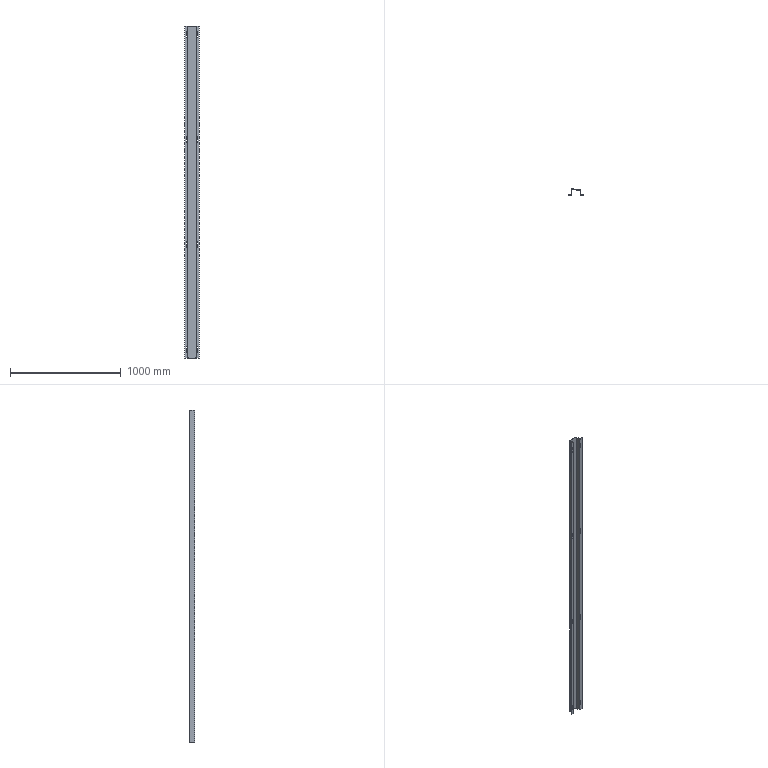Part | STEP file | SX-014-01 | 1 solid | 118 faces | box 134 x 49.886 x 2995 mm | volume 1979829 mm3 | plane 70 | cylinder 40 | spline 8 | commonest cylinder face diameters 6 x16 0.4 x12 6.4 x12